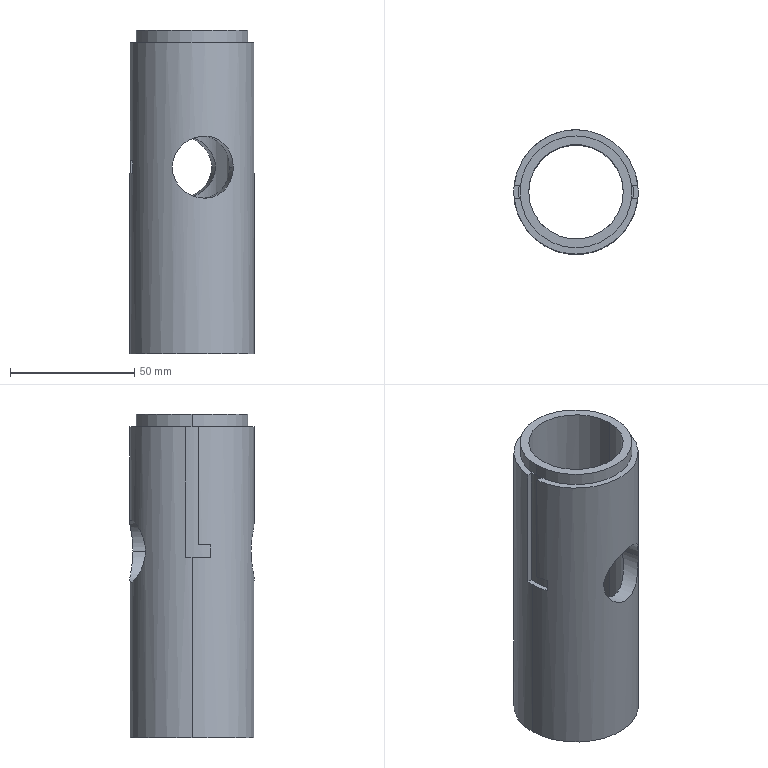Part | STEP file | Large bronze bushing SGN-2-27 | 1 solid | 26 faces | box 50 x 50 x 130 mm | volume 98629 mm3 | cylinder 13 | plane 13 | commonest cylinder face diameters 25 x4 46 x3 38 x2 45 x2 50 x2